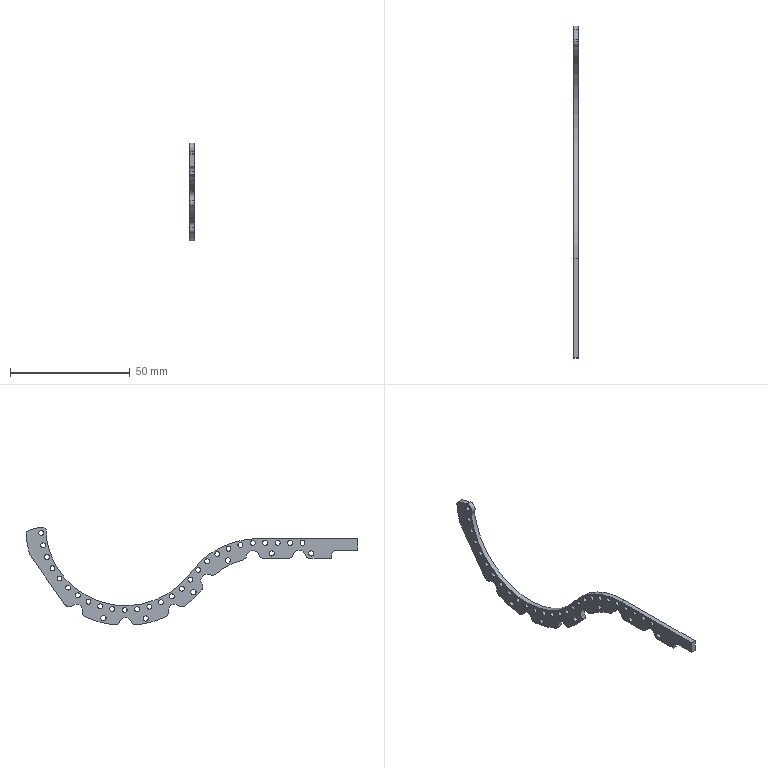Part | SolidWorks | features Extrusion 1, Fillet 1 | 1 solid | 119 faces | box 2 x 138.567 x 40.786 mm | volume 2138 mm3 | cylinder 109 | plane 10 | commonest cylinder face diameters 2.05 x54 4 x21 2.2 x12 5.2 x12 83.4 x5 4.8 x2